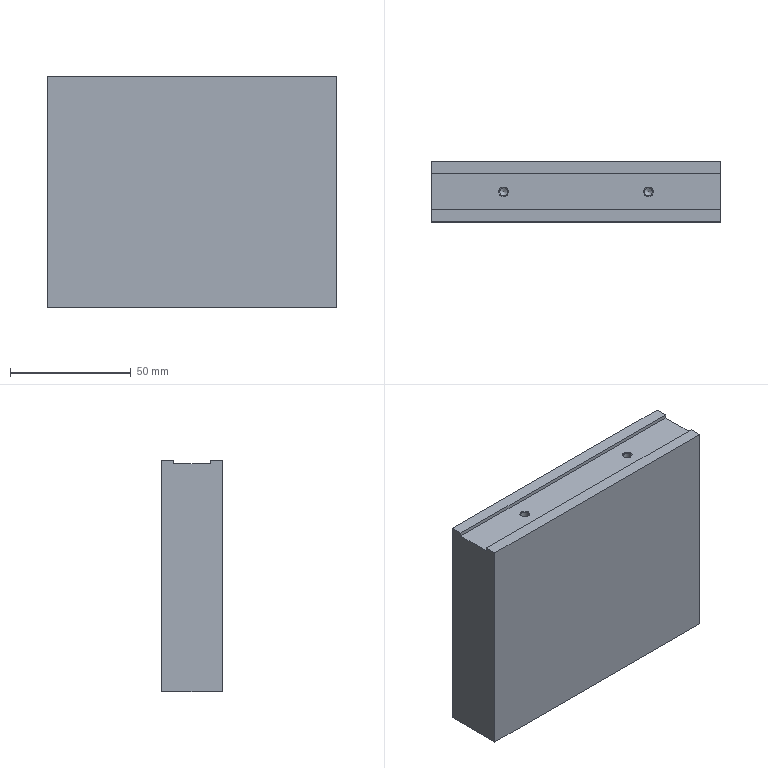Part | STEP file | Tube necking machine_id566_x_t | 1 solid | 16 faces | box 120 x 25 x 96 mm | volume 284951 mm3 | plane 10 | cone 4 | cylinder 2 | commonest cylinder face diameters 3.3 x2
STEP:
#1=CARTESIAN_POINT('',(0.,0.,0.));
#2=DIRECTION('',(0.,0.,1.));
#3=DIRECTION('',(1.,0.,0.));
#4=AXIS2_PLACEMENT_3D('',#1,#2,#3);
#5=CARTESIAN_POINT('',(210.,57.5,116.));
#6=VERTEX_POINT('',#5);
#7=CARTESIAN_POINT('',(210.,57.5,114.5));
#8=VERTEX_POINT('',#7);
#9=CARTESIAN_POINT('',(210.,57.5,115.681));
#10=DIRECTION('',(0.,0.,-1.));
#11=VECTOR('',#10,1.);
#12=LINE('',#9,#11);
#13=CARTESIAN_POINT('',(210.,62.5,136.));
#14=DIRECTION('',(1.,0.,0.));
#15=DIRECTION('',(0.,0.,-1.));
#16=AXIS2_PLACEMENT_3D('',#13,#14,#15);
#17=PLANE('',#16);
#18=CARTESIAN_POINT('',(20.319,-5.));
#19=DIRECTION('',(1.,0.));
#20=VECTOR('',#19,1.);
#21=LINE('',#18,#20);
#22=(GEOMETRIC_REPRESENTATION_CONTEXT(2)PARAMETRIC_REPRESENTATION_CONTEXT()REPRESENTATION_CONTEXT('',''));
#23=DEFINITIONAL_REPRESENTATION('',(#21),#22);
#24=PCURVE('',#17,#23);
#25=CARTESIAN_POINT('',(-741.73,57.5,115.681));
#26=DIRECTION('',(0.,1.,0.));
#27=DIRECTION('',(0.,0.,1.));
#28=AXIS2_PLACEMENT_3D('',#25,#26,#27);
#29=PLANE('',#28);
#30=CARTESIAN_POINT('',(0.,951.73));
#31=DIRECTION('',(-1.,0.));
#32=VECTOR('',#31,1.);
#33=LINE('',#30,#32);
#34=(GEOMETRIC_REPRESENTATION_CONTEXT(2)PARAMETRIC_REPRESENTATION_CONTEXT()REPRESENTATION_CONTEXT('',''));
#35=DEFINITIONAL_REPRESENTATION('',(#33),#34);
#36=PCURVE('',#29,#35);
#37=SURFACE_CURVE('',#12,(#24,#36),.PCURVE_S1.);
#38=EDGE_CURVE('',#6,#8,#37,.T.);
#39=ORIENTED_EDGE('',*,*,#38,.F.);
#40=CARTESIAN_POINT('',(210.,62.5,116.));
#41=VERTEX_POINT('',#40);
#42=CARTESIAN_POINT('',(210.,62.5,116.));
#43=DIRECTION('',(0.,-1.,0.));
#44=VECTOR('',#43,1.);
#45=LINE('',#42,#44);
#46=CARTESIAN_POINT('',(20.,0.));
#47=DIRECTION('',(0.,-1.));
#48=VECTOR('',#47,1.);
#49=LINE('',#46,#48);
#50=(GEOMETRIC_REPRESENTATION_CONTEXT(2)PARAMETRIC_REPRESENTATION_CONTEXT()REPRESENTATION_CONTEXT('',''));
#51=DEFINITIONAL_REPRESENTATION('',(#49),#50);
#52=PCURVE('',#17,#51);
#53=CARTESIAN_POINT('',(2.5,0.,116.));
#54=DIRECTION('',(0.,0.,1.));
#55=DIRECTION('',(1.,0.,0.));
#56=AXIS2_PLACEMENT_3D('',#53,#54,#55);
#57=PLANE('',#56);
#58=CARTESIAN_POINT('',(207.5,62.5));
#59=DIRECTION('',(0.,-1.));
#60=VECTOR('',#59,1.);
#61=LINE('',#58,#60);
#62=(GEOMETRIC_REPRESENTATION_CONTEXT(2)PARAMETRIC_REPRESENTATION_CONTEXT()REPRESENTATION_CONTEXT('',''));
#63=DEFINITIONAL_REPRESENTATION('',(#61),#62);
#64=PCURVE('',#57,#63);
#65=SURFACE_CURVE('',#45,(#52,#64),.PCURVE_S1.);
#66=EDGE_CURVE('',#41,#6,#65,.T.);
#67=ORIENTED_EDGE('',*,*,#66,.F.);
#68=CARTESIAN_POINT('',(210.,62.5,20.));
#69=VERTEX_POINT('',#68);
#70=CARTESIAN_POINT('',(210.,62.5,136.));
#71=DIRECTION('',(0.,0.,-1.));
#72=VECTOR('',#71,1.);
#73=LINE('',#70,#72);
#74=CARTESIAN_POINT('',(0.,0.));
#75=DIRECTION('',(1.,0.));
#76=VECTOR('',#75,1.);
#77=LINE('',#74,#76);
#78=(GEOMETRIC_REPRESENTATION_CONTEXT(2)PARAMETRIC_REPRESENTATION_CONTEXT()REPRESENTATION_CONTEXT('',''));
#79=DEFINITIONAL_REPRESENTATION('',(#77),#78);
#80=PCURVE('',#17,#79);
#81=CARTESIAN_POINT('',(330.,62.5,136.));
#82=DIRECTION('',(0.,-1.,0.));
#83=DIRECTION('',(0.,0.,-1.));
#84=AXIS2_PLACEMENT_3D('',#81,#82,#83);
#85=PLANE('',#84);
#86=CARTESIAN_POINT('',(0.,-120.));
#87=DIRECTION('',(1.,0.));
#88=VECTOR('',#87,1.);
#89=LINE('',#86,#88);
#90=(GEOMETRIC_REPRESENTATION_CONTEXT(2)PARAMETRIC_REPRESENTATION_CONTEXT()REPRESENTATION_CONTEXT('',''));
#91=DEFINITIONAL_REPRESENTATION('',(#89),#90);
#92=PCURVE('',#85,#91);
#93=SURFACE_CURVE('',#73,(#80,#92),.PCURVE_S1.);
#94=EDGE_CURVE('',#41,#69,#93,.T.);
#95=ORIENTED_EDGE('',*,*,#94,.T.);
#96=CARTESIAN_POINT('',(210.,37.5,20.));
#97=VERTEX_POINT('',#96);
#98=CARTESIAN_POINT('',(210.,62.5,20.));
#99=DIRECTION('',(0.,-1.,0.));
#100=VECTOR('',#99,1.);
#101=LINE('',#98,#100);
#102=CARTESIAN_POINT('',(116.,0.));
#103=DIRECTION('',(0.,-1.));
#104=VECTOR('',#103,1.);
#105=LINE('',#102,#104);
#106=(GEOMETRIC_REPRESENTATION_CONTEXT(2)PARAMETRIC_REPRESENTATION_CONTEXT()REPRESENTATION_CONTEXT('',''));
#107=DEFINITIONAL_REPRESENTATION('',(#105),#106);
#108=PCURVE('',#17,#107);
#109=CARTESIAN_POINT('',(2.5,0.,20.));
#110=DIRECTION('',(0.,0.,1.));
#111=DIRECTION('',(1.,0.,0.));
#112=AXIS2_PLACEMENT_3D('',#109,#110,#111);
#113=PLANE('',#112);
#114=CARTESIAN_POINT('',(207.5,62.5));
#115=DIRECTION('',(0.,-1.));
#116=VECTOR('',#115,1.);
#117=LINE('',#114,#116);
#118=(GEOMETRIC_REPRESENTATION_CONTEXT(2)PARAMETRIC_REPRESENTATION_CONTEXT()REPRESENTATION_CONTEXT('',''));
#119=DEFINITIONAL_REPRESENTATION('',(#117),#118);
#120=PCURVE('',#113,#119);
#121=SURFACE_CURVE('',#101,(#108,#120),.PCURVE_S1.);
#122=EDGE_CURVE('',#69,#97,#121,.T.);
#123=ORIENTED_EDGE('',*,*,#122,.T.);
#124=CARTESIAN_POINT('',(210.,37.5,116.));
#125=VERTEX_POINT('',#124);
#126=CARTESIAN_POINT('',(210.,37.5,136.));
#127=DIRECTION('',(0.,0.,-1.));
#128=VECTOR('',#127,1.);
#129=LINE('',#126,#128);
#130=CARTESIAN_POINT('',(0.,-25.));
#131=DIRECTION('',(1.,0.));
#132=VECTOR('',#131,1.);
#133=LINE('',#130,#132);
#134=(GEOMETRIC_REPRESENTATION_CONTEXT(2)PARAMETRIC_REPRESENTATION_CONTEXT()REPRESENTATION_CONTEXT('',''));
#135=DEFINITIONAL_REPRESENTATION('',(#133),#134);
#136=PCURVE('',#17,#135);
#137=CARTESIAN_POINT('',(210.,37.5,136.));
#138=DIRECTION('',(0.,1.,0.));
#139=DIRECTION('',(0.,0.,1.));
#140=AXIS2_PLACEMENT_3D('',#137,#138,#139);
#141=PLANE('',#140);
#142=CARTESIAN_POINT('',(0.,0.));
#143=DIRECTION('',(-1.,0.));
#144=VECTOR('',#143,1.);
#145=LINE('',#142,#144);
#146=(GEOMETRIC_REPRESENTATION_CONTEXT(2)PARAMETRIC_REPRESENTATION_CONTEXT()REPRESENTATION_CONTEXT('',''));
#147=DEFINITIONAL_REPRESENTATION('',(#145),#146);
#148=PCURVE('',#141,#147);
#149=SURFACE_CURVE('',#129,(#136,#148),.PCURVE_S1.);
#150=EDGE_CURVE('',#125,#97,#149,.T.);
#151=ORIENTED_EDGE('',*,*,#150,.F.);
#152=CARTESIAN_POINT('',(210.,42.5,116.));
#153=VERTEX_POINT('',#152);
#154=CARTESIAN_POINT('',(210.,62.5,116.));
#155=DIRECTION('',(0.,-1.,0.));
#156=VECTOR('',#155,1.);
#157=LINE('',#154,#156);
#158=CARTESIAN_POINT('',(20.,0.));
#159=DIRECTION('',(0.,-1.));
#160=VECTOR('',#159,1.);
#161=LINE('',#158,#160);
#162=(GEOMETRIC_REPRESENTATION_CONTEXT(2)PARAMETRIC_REPRESENTATION_CONTEXT()REPRESENTATION_CONTEXT('',''));
#163=DEFINITIONAL_REPRESENTATION('',(#161),#162);
#164=PCURVE('',#17,#163);
#165=CARTESIAN_POINT('',(2.5,0.,116.));
#166=DIRECTION('',(0.,0.,1.));
#167=DIRECTION('',(1.,0.,0.));
#168=AXIS2_PLACEMENT_3D('',#165,#166,#167);
#169=PLANE('',#168);
#170=CARTESIAN_POINT('',(207.5,62.5));
#171=DIRECTION('',(0.,-1.));
#172=VECTOR('',#171,1.);
#173=LINE('',#170,#172);
#174=(GEOMETRIC_REPRESENTATION_CONTEXT(2)PARAMETRIC_REPRESENTATION_CONTEXT()REPRESENTATION_CONTEXT('',''));
#175=DEFINITIONAL_REPRESENTATION('',(#173),#174);
#176=PCURVE('',#169,#175);
#177=SURFACE_CURVE('',#157,(#164,#176),.PCURVE_S1.);
#178=EDGE_CURVE('',#153,#125,#177,.T.);
#179=ORIENTED_EDGE('',*,*,#178,.F.);
#180=CARTESIAN_POINT('',(210.,42.5,114.5));
#181=VERTEX_POINT('',#180);
#182=CARTESIAN_POINT('',(210.,42.5,114.5));
#183=DIRECTION('',(0.,0.,1.));
#184=VECTOR('',#183,1.);
#185=LINE('',#182,#184);
#186=CARTESIAN_POINT('',(21.5,-20.));
#187=DIRECTION('',(-1.,0.));
#188=VECTOR('',#187,1.);
#189=LINE('',#186,#188);
#190=(GEOMETRIC_REPRESENTATION_CONTEXT(2)PARAMETRIC_REPRESENTATION_CONTEXT()REPRESENTATION_CONTEXT('',''));
#191=DEFINITIONAL_REPRESENTATION('',(#189),#190);
#192=PCURVE('',#17,#191);
#193=CARTESIAN_POINT('',(-741.73,42.5,114.5));
#194=DIRECTION('',(0.,-1.,0.));
#195=DIRECTION('',(0.,0.,-1.));
#196=AXIS2_PLACEMENT_3D('',#193,#194,#195);
#197=PLANE('',#196);
#198=CARTESIAN_POINT('',(0.,951.73));
#199=DIRECTION('',(-1.,0.));
#200=VECTOR('',#199,1.);
#201=LINE('',#198,#200);
#202=(GEOMETRIC_REPRESENTATION_CONTEXT(2)PARAMETRIC_REPRESENTATION_CONTEXT()REPRESENTATION_CONTEXT('',''));
#203=DEFINITIONAL_REPRESENTATION('',(#201),#202);
#204=PCURVE('',#197,#203);
#205=SURFACE_CURVE('',#185,(#192,#204),.PCURVE_S1.);
#206=EDGE_CURVE('',#181,#153,#205,.T.);
#207=ORIENTED_EDGE('',*,*,#206,.F.);
#208=CARTESIAN_POINT('',(210.,57.5,114.5));
#209=DIRECTION('',(0.,-1.,0.));
#210=VECTOR('',#209,1.);
#211=LINE('',#208,#210);
#212=CARTESIAN_POINT('',(21.5,-5.));
#213=DIRECTION('',(0.,-1.));
#214=VECTOR('',#213,1.);
#215=LINE('',#212,#214);
#216=(GEOMETRIC_REPRESENTATION_CONTEXT(2)PARAMETRIC_REPRESENTATION_CONTEXT()REPRESENTATION_CONTEXT('',''));
#217=DEFINITIONAL_REPRESENTATION('',(#215),#216);
#218=PCURVE('',#17,#217);
#219=CARTESIAN_POINT('',(-741.73,57.5,114.5));
#220=DIRECTION('',(0.,0.,-1.));
#221=DIRECTION('',(1.,0.,0.));
#222=AXIS2_PLACEMENT_3D('',#219,#220,#221);
#223=PLANE('',#222);
#224=CARTESIAN_POINT('',(951.73,0.));
#225=DIRECTION('',(0.,1.));
#226=VECTOR('',#225,1.);
#227=LINE('',#224,#226);
#228=(GEOMETRIC_REPRESENTATION_CONTEXT(2)PARAMETRIC_REPRESENTATION_CONTEXT()REPRESENTATION_CONTEXT('',''));
#229=DEFINITIONAL_REPRESENTATION('',(#227),#228);
#230=PCURVE('',#223,#229);
#231=SURFACE_CURVE('',#211,(#218,#230),.PCURVE_S1.);
#232=EDGE_CURVE('',#8,#181,#231,.T.);
#233=ORIENTED_EDGE('',*,*,#232,.F.);
#234=EDGE_LOOP('',(#39,#67,#95,#123,#151,#179,#207,#233));
#235=FACE_BOUND('',#234,.T.);
#236=ADVANCED_FACE('',(#235),#17,.F.);
#237=CARTESIAN_POINT('',(330.,42.5,116.));
#238=VERTEX_POINT('',#237);
#239=CARTESIAN_POINT('',(330.,42.5,114.5));
#240=VERTEX_POINT('',#239);
#241=CARTESIAN_POINT('',(330.,42.5,114.5));
#242=DIRECTION('',(0.,0.,-1.));
#243=VECTOR('',#242,1.);
#244=LINE('',#241,#243);
#245=CARTESIAN_POINT('',(330.,37.5,136.));
#246=DIRECTION('',(-1.,0.,0.));
#247=DIRECTION('',(0.,0.,1.));
#248=AXIS2_PLACEMENT_3D('',#245,#246,#247);
#249=PLANE('',#248);
#250=CARTESIAN_POINT('',(-21.5,5.));
#251=DIRECTION('',(-1.,0.));
#252=VECTOR('',#251,1.);
#253=LINE('',#250,#252);
#254=(GEOMETRIC_REPRESENTATION_CONTEXT(2)PARAMETRIC_REPRESENTATION_CONTEXT()REPRESENTATION_CONTEXT('',''));
#255=DEFINITIONAL_REPRESENTATION('',(#253),#254);
#256=PCURVE('',#249,#255);
#257=CARTESIAN_POINT('',(0.,1071.73));
#258=DIRECTION('',(1.,0.));
#259=VECTOR('',#258,1.);
#260=LINE('',#257,#259);
#261=(GEOMETRIC_REPRESENTATION_CONTEXT(2)PARAMETRIC_REPRESENTATION_CONTEXT()REPRESENTATION_CONTEXT('',''));
#262=DEFINITIONAL_REPRESENTATION('',(#260),#261);
#263=PCURVE('',#197,#262);
#264=SURFACE_CURVE('',#244,(#256,#263),.PCURVE_S1.);
#265=EDGE_CURVE('',#238,#240,#264,.T.);
#266=ORIENTED_EDGE('',*,*,#265,.F.);
#267=CARTESIAN_POINT('',(330.,37.5,116.));
#268=VERTEX_POINT('',#267);
#269=CARTESIAN_POINT('',(330.,37.5,116.));
#270=DIRECTION('',(0.,1.,0.));
#271=VECTOR('',#270,1.);
#272=LINE('',#269,#271);
#273=CARTESIAN_POINT('',(-20.,0.));
#274=DIRECTION('',(0.,1.));
#275=VECTOR('',#274,1.);
#276=LINE('',#273,#275);
#277=(GEOMETRIC_REPRESENTATION_CONTEXT(2)PARAMETRIC_REPRESENTATION_CONTEXT()REPRESENTATION_CONTEXT('',''));
#278=DEFINITIONAL_REPRESENTATION('',(#276),#277);
#279=PCURVE('',#249,#278);
#280=CARTESIAN_POINT('',(327.5,37.5));
#281=DIRECTION('',(0.,1.));
#282=VECTOR('',#281,1.);
#283=LINE('',#280,#282);
#284=(GEOMETRIC_REPRESENTATION_CONTEXT(2)PARAMETRIC_REPRESENTATION_CONTEXT()REPRESENTATION_CONTEXT('',''));
#285=DEFINITIONAL_REPRESENTATION('',(#283),#284);
#286=PCURVE('',#169,#285);
#287=SURFACE_CURVE('',#272,(#279,#286),.PCURVE_S1.);
#288=EDGE_CURVE('',#268,#238,#287,.T.);
#289=ORIENTED_EDGE('',*,*,#288,.F.);
#290=CARTESIAN_POINT('',(330.,37.5,20.));
#291=VERTEX_POINT('',#290);
#292=CARTESIAN_POINT('',(330.,37.5,136.));
#293=DIRECTION('',(0.,0.,-1.));
#294=VECTOR('',#293,1.);
#295=LINE('',#292,#294);
#296=CARTESIAN_POINT('',(0.,0.));
#297=DIRECTION('',(-1.,0.));
#298=VECTOR('',#297,1.);
#299=LINE('',#296,#298);
#300=(GEOMETRIC_REPRESENTATION_CONTEXT(2)PARAMETRIC_REPRESENTATION_CONTEXT()REPRESENTATION_CONTEXT('',''));
#301=DEFINITIONAL_REPRESENTATION('',(#299),#300);
#302=PCURVE('',#249,#301);
#303=CARTESIAN_POINT('',(0.,120.));
#304=DIRECTION('',(-1.,0.));
#305=VECTOR('',#304,1.);
#306=LINE('',#303,#305);
#307=(GEOMETRIC_REPRESENTATION_CONTEXT(2)PARAMETRIC_REPRESENTATION_CONTEXT()REPRESENTATION_CONTEXT('',''));
#308=DEFINITIONAL_REPRESENTATION('',(#306),#307);
#309=PCURVE('',#141,#308);
#310=SURFACE_CURVE('',#295,(#302,#309),.PCURVE_S1.);
#311=EDGE_CURVE('',#268,#291,#310,.T.);
#312=ORIENTED_EDGE('',*,*,#311,.T.);
#313=CARTESIAN_POINT('',(330.,62.5,20.));
#314=VERTEX_POINT('',#313);
#315=CARTESIAN_POINT('',(330.,37.5,20.));
#316=DIRECTION('',(0.,1.,0.));
#317=VECTOR('',#316,1.);
#318=LINE('',#315,#317);
#319=CARTESIAN_POINT('',(-116.,0.));
#320=DIRECTION('',(0.,1.));
#321=VECTOR('',#320,1.);
#322=LINE('',#319,#321);
#323=(GEOMETRIC_REPRESENTATION_CONTEXT(2)PARAMETRIC_REPRESENTATION_CONTEXT()REPRESENTATION_CONTEXT('',''));
#324=DEFINITIONAL_REPRESENTATION('',(#322),#323);
#325=PCURVE('',#249,#324);
#326=CARTESIAN_POINT('',(327.5,37.5));
#327=DIRECTION('',(0.,1.));
#328=VECTOR('',#327,1.);
#329=LINE('',#326,#328);
#330=(GEOMETRIC_REPRESENTATION_CONTEXT(2)PARAMETRIC_REPRESENTATION_CONTEXT()REPRESENTATION_CONTEXT('',''));
#331=DEFINITIONAL_REPRESENTATION('',(#329),#330);
#332=PCURVE('',#113,#331);
#333=SURFACE_CURVE('',#318,(#325,#332),.PCURVE_S1.);
#334=EDGE_CURVE('',#291,#314,#333,.T.);
#335=ORIENTED_EDGE('',*,*,#334,.T.);
#336=CARTESIAN_POINT('',(330.,62.5,116.));
#337=VERTEX_POINT('',#336);
#338=CARTESIAN_POINT('',(330.,62.5,136.));
#339=DIRECTION('',(0.,0.,-1.));
#340=VECTOR('',#339,1.);
#341=LINE('',#338,#340);
#342=CARTESIAN_POINT('',(0.,25.));
#343=DIRECTION('',(-1.,0.));
#344=VECTOR('',#343,1.);
#345=LINE('',#342,#344);
#346=(GEOMETRIC_REPRESENTATION_CONTEXT(2)PARAMETRIC_REPRESENTATION_CONTEXT()REPRESENTATION_CONTEXT('',''));
#347=DEFINITIONAL_REPRESENTATION('',(#345),#346);
#348=PCURVE('',#249,#347);
#349=CARTESIAN_POINT('',(0.,0.));
#350=DIRECTION('',(1.,0.));
#351=VECTOR('',#350,1.);
#352=LINE('',#349,#351);
#353=(GEOMETRIC_REPRESENTATION_CONTEXT(2)PARAMETRIC_REPRESENTATION_CONTEXT()REPRESENTATION_CONTEXT('',''));
#354=DEFINITIONAL_REPRESENTATION('',(#352),#353);
#355=PCURVE('',#85,#354);
#356=SURFACE_CURVE('',#341,(#348,#355),.PCURVE_S1.);
#357=EDGE_CURVE('',#337,#314,#356,.T.);
#358=ORIENTED_EDGE('',*,*,#357,.F.);
#359=CARTESIAN_POINT('',(330.,57.5,116.));
#360=VERTEX_POINT('',#359);
#361=CARTESIAN_POINT('',(330.,37.5,116.));
#362=DIRECTION('',(0.,1.,0.));
#363=VECTOR('',#362,1.);
#364=LINE('',#361,#363);
#365=CARTESIAN_POINT('',(-20.,0.));
#366=DIRECTION('',(0.,1.));
#367=VECTOR('',#366,1.);
#368=LINE('',#365,#367);
#369=(GEOMETRIC_REPRESENTATION_CONTEXT(2)PARAMETRIC_REPRESENTATION_CONTEXT()REPRESENTATION_CONTEXT('',''));
#370=DEFINITIONAL_REPRESENTATION('',(#368),#369);
#371=PCURVE('',#249,#370);
#372=CARTESIAN_POINT('',(327.5,37.5));
#373=DIRECTION('',(0.,1.));
#374=VECTOR('',#373,1.);
#375=LINE('',#372,#374);
#376=(GEOMETRIC_REPRESENTATION_CONTEXT(2)PARAMETRIC_REPRESENTATION_CONTEXT()REPRESENTATION_CONTEXT('',''));
#377=DEFINITIONAL_REPRESENTATION('',(#375),#376);
#378=PCURVE('',#57,#377);
#379=SURFACE_CURVE('',#364,(#371,#378),.PCURVE_S1.);
#380=EDGE_CURVE('',#360,#337,#379,.T.);
#381=ORIENTED_EDGE('',*,*,#380,.F.);
#382=CARTESIAN_POINT('',(330.,57.5,114.5));
#383=VERTEX_POINT('',#382);
#384=CARTESIAN_POINT('',(330.,57.5,115.681));
#385=DIRECTION('',(0.,0.,1.));
#386=VECTOR('',#385,1.);
#387=LINE('',#384,#386);
#388=CARTESIAN_POINT('',(-20.319,20.));
#389=DIRECTION('',(1.,0.));
#390=VECTOR('',#389,1.);
#391=LINE('',#388,#390);
#392=(GEOMETRIC_REPRESENTATION_CONTEXT(2)PARAMETRIC_REPRESENTATION_CONTEXT()REPRESENTATION_CONTEXT('',''));
#393=DEFINITIONAL_REPRESENTATION('',(#391),#392);
#394=PCURVE('',#249,#393);
#395=CARTESIAN_POINT('',(0.,1071.73));
#396=DIRECTION('',(1.,0.));
#397=VECTOR('',#396,1.);
#398=LINE('',#395,#397);
#399=(GEOMETRIC_REPRESENTATION_CONTEXT(2)PARAMETRIC_REPRESENTATION_CONTEXT()REPRESENTATION_CONTEXT('',''));
#400=DEFINITIONAL_REPRESENTATION('',(#398),#399);
#401=PCURVE('',#29,#400);
#402=SURFACE_CURVE('',#387,(#394,#401),.PCURVE_S1.);
#403=EDGE_CURVE('',#383,#360,#402,.T.);
#404=ORIENTED_EDGE('',*,*,#403,.F.);
#405=CARTESIAN_POINT('',(330.,57.5,114.5));
#406=DIRECTION('',(0.,1.,0.));
#407=VECTOR('',#406,1.);
#408=LINE('',#405,#407);
#409=CARTESIAN_POINT('',(-21.5,20.));
#410=DIRECTION('',(0.,1.));
#411=VECTOR('',#410,1.);
#412=LINE('',#409,#411);
#413=(GEOMETRIC_REPRESENTATION_CONTEXT(2)PARAMETRIC_REPRESENTATION_CONTEXT()REPRESENTATION_CONTEXT('',''));
#414=DEFINITIONAL_REPRESENTATION('',(#412),#413);
#415=PCURVE('',#249,#414);
#416=CARTESIAN_POINT('',(1071.73,0.));
#417=DIRECTION('',(0.,-1.));
#418=VECTOR('',#417,1.);
#419=LINE('',#416,#418);
#420=(GEOMETRIC_REPRESENTATION_CONTEXT(2)PARAMETRIC_REPRESENTATION_CONTEXT()REPRESENTATION_CONTEXT('',''));
#421=DEFINITIONAL_REPRESENTATION('',(#419),#420);
#422=PCURVE('',#223,#421);
#423=SURFACE_CURVE('',#408,(#415,#422),.PCURVE_S1.);
#424=EDGE_CURVE('',#240,#383,#423,.T.);
#425=ORIENTED_EDGE('',*,*,#424,.F.);
#426=EDGE_LOOP('',(#266,#289,#312,#335,#358,#381,#404,#425));
#427=FACE_BOUND('',#426,.T.);
#428=ADVANCED_FACE('',(#427),#249,.F.);
#429=CARTESIAN_POINT('',(2.5,42.5,116.));
#430=DIRECTION('',(1.,0.,0.));
#431=VECTOR('',#430,1.);
#432=LINE('',#429,#431);
#433=CARTESIAN_POINT('',(0.,42.5));
#434=DIRECTION('',(1.,0.));
#435=VECTOR('',#434,1.);
#436=LINE('',#433,#435);
#437=(GEOMETRIC_REPRESENTATION_CONTEXT(2)PARAMETRIC_REPRESENTATION_CONTEXT()REPRESENTATION_CONTEXT('',''));
#438=DEFINITIONAL_REPRESENTATION('',(#436),#437);
#439=PCURVE('',#169,#438);
#440=CARTESIAN_POINT('',(-1.5,744.23));
#441=DIRECTION('',(0.,1.));
#442=VECTOR('',#441,1.);
#443=LINE('',#440,#442);
#444=(GEOMETRIC_REPRESENTATION_CONTEXT(2)PARAMETRIC_REPRESENTATION_CONTEXT()REPRESENTATION_CONTEXT('',''));
#445=DEFINITIONAL_REPRESENTATION('',(#443),#444);
#446=PCURVE('',#197,#445);
#447=SURFACE_CURVE('',#432,(#439,#446),.PCURVE_S1.);
#448=EDGE_CURVE('',#153,#238,#447,.T.);
#449=ORIENTED_EDGE('',*,*,#448,.F.);
#450=ORIENTED_EDGE('',*,*,#178,.T.);
#451=CARTESIAN_POINT('',(210.,37.5,116.));
#452=DIRECTION('',(1.,0.,0.));
#453=VECTOR('',#452,1.);
#454=LINE('',#451,#453);
#455=CARTESIAN_POINT('',(207.5,37.5));
#456=DIRECTION('',(1.,0.));
#457=VECTOR('',#456,1.);
#458=LINE('',#455,#457);
#459=(GEOMETRIC_REPRESENTATION_CONTEXT(2)PARAMETRIC_REPRESENTATION_CONTEXT()REPRESENTATION_CONTEXT('',''));
#460=DEFINITIONAL_REPRESENTATION('',(#458),#459);
#461=PCURVE('',#169,#460);
#462=CARTESIAN_POINT('',(-20.,0.));
#463=DIRECTION('',(0.,1.));
#464=VECTOR('',#463,1.);
#465=LINE('',#462,#464);
#466=(GEOMETRIC_REPRESENTATION_CONTEXT(2)PARAMETRIC_REPRESENTATION_CONTEXT()REPRESENTATION_CONTEXT('',''));
#467=DEFINITIONAL_REPRESENTATION('',(#465),#466);
#468=PCURVE('',#141,#467);
#469=SURFACE_CURVE('',#454,(#461,#468),.PCURVE_S1.);
#470=EDGE_CURVE('',#125,#268,#469,.T.);
#471=ORIENTED_EDGE('',*,*,#470,.T.);
#472=ORIENTED_EDGE('',*,*,#288,.T.);
#473=EDGE_LOOP('',(#449,#450,#471,#472));
#474=FACE_BOUND('',#473,.T.);
#475=ADVANCED_FACE('',(#474),#169,.T.);
#476=ORIENTED_EDGE('',*,*,#470,.F.);
#477=ORIENTED_EDGE('',*,*,#150,.T.);
#478=CARTESIAN_POINT('',(210.,37.5,20.));
#479=DIRECTION('',(1.,0.,0.));
#480=VECTOR('',#479,1.);
#481=LINE('',#478,#480);
#482=CARTESIAN_POINT('',(-116.,0.));
#483=DIRECTION('',(0.,1.));
#484=VECTOR('',#483,1.);
#485=LINE('',#482,#484);
#486=(GEOMETRIC_REPRESENTATION_CONTEXT(2)PARAMETRIC_REPRESENTATION_CONTEXT()REPRESENTATION_CONTEXT('',''));
#487=DEFINITIONAL_REPRESENTATION('',(#485),#486);
#488=PCURVE('',#141,#487);
#489=CARTESIAN_POINT('',(207.5,37.5));
#490=DIRECTION('',(1.,0.));
#491=VECTOR('',#490,1.);
#492=LINE('',#489,#491);
#493=(GEOMETRIC_REPRESENTATION_CONTEXT(2)PARAMETRIC_REPRESENTATION_CONTEXT()REPRESENTATION_CONTEXT('',''));
#494=DEFINITIONAL_REPRESENTATION('',(#492),#493);
#495=PCURVE('',#113,#494);
#496=SURFACE_CURVE('',#481,(#488,#495),.PCURVE_S1.);
#497=EDGE_CURVE('',#97,#291,#496,.T.);
#498=ORIENTED_EDGE('',*,*,#497,.T.);
#499=ORIENTED_EDGE('',*,*,#311,.F.);
#500=EDGE_LOOP('',(#476,#477,#498,#499));
#501=FACE_BOUND('',#500,.T.);
#502=ADVANCED_FACE('',(#501),#141,.F.);
#503=CARTESIAN_POINT('',(330.,62.5,116.));
#504=DIRECTION('',(-1.,0.,0.));
#505=VECTOR('',#504,1.);
#506=LINE('',#503,#505);
#507=CARTESIAN_POINT('',(20.,0.));
#508=DIRECTION('',(0.,-1.));
#509=VECTOR('',#508,1.);
#510=LINE('',#507,#509);
#511=(GEOMETRIC_REPRESENTATION_CONTEXT(2)PARAMETRIC_REPRESENTATION_CONTEXT()REPRESENTATION_CONTEXT('',''));
#512=DEFINITIONAL_REPRESENTATION('',(#510),#511);
#513=PCURVE('',#85,#512);
#514=CARTESIAN_POINT('',(327.5,62.5));
#515=DIRECTION('',(-1.,0.));
#516=VECTOR('',#515,1.);
#517=LINE('',#514,#516);
#518=(GEOMETRIC_REPRESENTATION_CONTEXT(2)PARAMETRIC_REPRESENTATION_CONTEXT()REPRESENTATION_CONTEXT('',''));
#519=DEFINITIONAL_REPRESENTATION('',(#517),#518);
#520=PCURVE('',#57,#519);
#521=SURFACE_CURVE('',#506,(#513,#520),.PCURVE_S1.);
#522=EDGE_CURVE('',#337,#41,#521,.T.);
#523=ORIENTED_EDGE('',*,*,#522,.F.);
#524=ORIENTED_EDGE('',*,*,#357,.T.);
#525=CARTESIAN_POINT('',(330.,62.5,20.));
#526=DIRECTION('',(-1.,0.,0.));
#527=VECTOR('',#526,1.);
#528=LINE('',#525,#527);
#529=CARTESIAN_POINT('',(116.,0.));
#530=DIRECTION('',(0.,-1.));
#531=VECTOR('',#530,1.);
#532=LINE('',#529,#531);
#533=(GEOMETRIC_REPRESENTATION_CONTEXT(2)PARAMETRIC_REPRESENTATION_CONTEXT()REPRESENTATION_CONTEXT('',''));
#534=DEFINITIONAL_REPRESENTATION('',(#532),#533);
#535=PCURVE('',#85,#534);
#536=CARTESIAN_POINT('',(327.5,62.5));
#537=DIRECTION('',(-1.,0.));
#538=VECTOR('',#537,1.);
#539=LINE('',#536,#538);
#540=(GEOMETRIC_REPRESENTATION_CONTEXT(2)PARAMETRIC_REPRESENTATION_CONTEXT()REPRESENTATION_CONTEXT('',''));
#541=DEFINITIONAL_REPRESENTATION('',(#539),#540);
#542=PCURVE('',#113,#541);
#543=SURFACE_CURVE('',#528,(#535,#542),.PCURVE_S1.);
#544=EDGE_CURVE('',#314,#69,#543,.T.);
#545=ORIENTED_EDGE('',*,*,#544,.T.);
#546=ORIENTED_EDGE('',*,*,#94,.F.);
#547=EDGE_LOOP('',(#523,#524,#545,#546));
#548=FACE_BOUND('',#547,.T.);
#549=ADVANCED_FACE('',(#548),#85,.F.);
#550=ORIENTED_EDGE('',*,*,#122,.F.);
#551=ORIENTED_EDGE('',*,*,#544,.F.);
#552=ORIENTED_EDGE('',*,*,#334,.F.);
#553=ORIENTED_EDGE('',*,*,#497,.F.);
#554=EDGE_LOOP('',(#550,#551,#552,#553));
#555=FACE_BOUND('',#554,.T.);
#556=ADVANCED_FACE('',(#555),#113,.F.);
#557=CARTESIAN_POINT('',(2.5,57.5,116.));
#558=DIRECTION('',(-1.,0.,0.));
#559=VECTOR('',#558,1.);
#560=LINE('',#557,#559);
#561=CARTESIAN_POINT('',(0.,57.5));
#562=DIRECTION('',(-1.,0.));
#563=VECTOR('',#562,1.);
#564=LINE('',#561,#563);
#565=(GEOMETRIC_REPRESENTATION_CONTEXT(2)PARAMETRIC_REPRESENTATION_CONTEXT()REPRESENTATION_CONTEXT('',''));
#566=DEFINITIONAL_REPRESENTATION('',(#564),#565);
#567=PCURVE('',#57,#566);
#568=CARTESIAN_POINT('',(0.3185,744.23));
#569=DIRECTION('',(0.,-1.));
#570=VECTOR('',#569,1.);
#571=LINE('',#568,#570);
#572=(GEOMETRIC_REPRESENTATION_CONTEXT(2)PARAMETRIC_REPRESENTATION_CONTEXT()REPRESENTATION_CONTEXT('',''));
#573=DEFINITIONAL_REPRESENTATION('',(#571),#572);
#574=PCURVE('',#29,#573);
#575=SURFACE_CURVE('',#560,(#567,#574),.PCURVE_S1.);
#576=EDGE_CURVE('',#360,#6,#575,.T.);
#577=ORIENTED_EDGE('',*,*,#576,.F.);
#578=ORIENTED_EDGE('',*,*,#380,.T.);
#579=ORIENTED_EDGE('',*,*,#522,.T.);
#580=ORIENTED_EDGE('',*,*,#66,.T.);
#581=EDGE_LOOP('',(#577,#578,#579,#580));
#582=FACE_BOUND('',#581,.T.);
#583=ADVANCED_FACE('',(#582),#57,.T.);
#584=ORIENTED_EDGE('',*,*,#448,.T.);
#585=ORIENTED_EDGE('',*,*,#265,.T.);
#586=CARTESIAN_POINT('',(-741.73,42.5,114.5));
#587=DIRECTION('',(1.,0.,0.));
#588=VECTOR('',#587,1.);
#589=LINE('',#586,#588);
#590=CARTESIAN_POINT('',(0.,0.));
#591=DIRECTION('',(0.,1.));
#592=VECTOR('',#591,1.);
#593=LINE('',#590,#592);
#594=(GEOMETRIC_REPRESENTATION_CONTEXT(2)PARAMETRIC_REPRESENTATION_CONTEXT()REPRESENTATION_CONTEXT('',''));
#595=DEFINITIONAL_REPRESENTATION('',(#593),#594);
#596=PCURVE('',#197,#595);
#597=CARTESIAN_POINT('',(0.,15.));
#598=DIRECTION('',(1.,0.));
#599=VECTOR('',#598,1.);
#600=LINE('',#597,#599);
#601=(GEOMETRIC_REPRESENTATION_CONTEXT(2)PARAMETRIC_REPRESENTATION_CONTEXT()REPRESENTATION_CONTEXT('',''));
#602=DEFINITIONAL_REPRESENTATION('',(#600),#601);
#603=PCURVE('',#223,#602);
#604=SURFACE_CURVE('',#589,(#596,#603),.PCURVE_S1.);
#605=EDGE_CURVE('',#181,#240,#604,.T.);
#606=ORIENTED_EDGE('',*,*,#605,.F.);
#607=ORIENTED_EDGE('',*,*,#206,.T.);
#608=EDGE_LOOP('',(#584,#585,#606,#607));
#609=FACE_BOUND('',#608,.T.);
#610=ADVANCED_FACE('',(#609),#197,.F.);
#611=ORIENTED_EDGE('',*,*,#576,.T.);
#612=ORIENTED_EDGE('',*,*,#38,.T.);
#613=CARTESIAN_POINT('',(-741.73,57.5,114.5));
#614=DIRECTION('',(1.,0.,0.));
#615=VECTOR('',#614,1.);
#616=LINE('',#613,#615);
#617=CARTESIAN_POINT('',(-1.181,0.));
#618=DIRECTION('',(0.,1.));
#619=VECTOR('',#618,1.);
#620=LINE('',#617,#619);
#621=(GEOMETRIC_REPRESENTATION_CONTEXT(2)PARAMETRIC_REPRESENTATION_CONTEXT()REPRESENTATION_CONTEXT('',''));
#622=DEFINITIONAL_REPRESENTATION('',(#620),#621);
#623=PCURVE('',#29,#622);
#624=CARTESIAN_POINT('',(0.,0.));
#625=DIRECTION('',(1.,0.));
#626=VECTOR('',#625,1.);
#627=LINE('',#624,#626);
#628=(GEOMETRIC_REPRESENTATION_CONTEXT(2)PARAMETRIC_REPRESENTATION_CONTEXT()REPRESENTATION_CONTEXT('',''));
#629=DEFINITIONAL_REPRESENTATION('',(#627),#628);
#630=PCURVE('',#223,#629);
#631=SURFACE_CURVE('',#616,(#623,#630),.PCURVE_S1.);
#632=EDGE_CURVE('',#8,#383,#631,.T.);
#633=ORIENTED_EDGE('',*,*,#632,.T.);
#634=ORIENTED_EDGE('',*,*,#403,.T.);
#635=EDGE_LOOP('',(#611,#612,#633,#634));
#636=FACE_BOUND('',#635,.T.);
#637=ADVANCED_FACE('',(#636),#29,.F.);
#638=CARTESIAN_POINT('',(298.,50.,114.5));
#639=VERTEX_POINT('',#638);
#640=CARTESIAN_POINT('',(300.,50.,114.5));
#641=DIRECTION('',(0.,0.,-1.));
#642=DIRECTION('',(-1.,0.,0.));
#643=AXIS2_PLACEMENT_3D('',#640,#641,#642);
#644=CIRCLE('',#643,2.);
#645=CARTESIAN_POINT('',(1041.73,7.5));
#646=DIRECTION('',(-1.,0.));
#647=AXIS2_PLACEMENT_2D('',#645,#646);
#648=CIRCLE('',#647,2.);
#649=(GEOMETRIC_REPRESENTATION_CONTEXT(2)PARAMETRIC_REPRESENTATION_CONTEXT()REPRESENTATION_CONTEXT('',''));
#650=DEFINITIONAL_REPRESENTATION('',(#648),#649);
#651=PCURVE('',#223,#650);
#652=CARTESIAN_POINT('',(300.,50.,114.5));
#653=DIRECTION('',(0.,0.,1.));
#654=DIRECTION('',(1.,0.,0.));
#655=AXIS2_PLACEMENT_3D('',#652,#653,#654);
#656=CONICAL_SURFACE('',#655,2.,0.7854);
#657=CARTESIAN_POINT('',(9.425,0.));
#658=DIRECTION('',(-1.,0.));
#659=VECTOR('',#658,1.);
#660=LINE('',#657,#659);
#661=(GEOMETRIC_REPRESENTATION_CONTEXT(2)PARAMETRIC_REPRESENTATION_CONTEXT()REPRESENTATION_CONTEXT('',''));
#662=DEFINITIONAL_REPRESENTATION('',(#660),#661);
#663=PCURVE('',#656,#662);
#664=SURFACE_CURVE('',#644,(#651,#663),.PCURVE_S1.);
#665=EDGE_CURVE('',#639,#639,#664,.T.);
#666=ORIENTED_EDGE('',*,*,#665,.T.);
#667=EDGE_LOOP('',(#666));
#668=FACE_BOUND('',#667,.T.);
#669=CARTESIAN_POINT('',(238.,50.,114.5));
#670=VERTEX_POINT('',#669);
#671=CARTESIAN_POINT('',(240.,50.,114.5));
#672=DIRECTION('',(0.,0.,-1.));
#673=DIRECTION('',(-1.,0.,0.));
#674=AXIS2_PLACEMENT_3D('',#671,#672,#673);
#675=CIRCLE('',#674,2.);
#676=CARTESIAN_POINT('',(981.73,7.5));
#677=DIRECTION('',(-1.,0.));
#678=AXIS2_PLACEMENT_2D('',#676,#677);
#679=CIRCLE('',#678,2.);
#680=(GEOMETRIC_REPRESENTATION_CONTEXT(2)PARAMETRIC_REPRESENTATION_CONTEXT()REPRESENTATION_CONTEXT('',''));
#681=DEFINITIONAL_REPRESENTATION('',(#679),#680);
#682=PCURVE('',#223,#681);
#683=CARTESIAN_POINT('',(240.,50.,114.5));
#684=DIRECTION('',(0.,0.,1.));
#685=DIRECTION('',(1.,0.,0.));
#686=AXIS2_PLACEMENT_3D('',#683,#684,#685);
#687=CONICAL_SURFACE('',#686,2.,0.7854);
#688=CARTESIAN_POINT('',(9.425,0.));
#689=DIRECTION('',(-1.,0.));
#690=VECTOR('',#689,1.);
#691=LINE('',#688,#690);
#692=(GEOMETRIC_REPRESENTATION_CONTEXT(2)PARAMETRIC_REPRESENTATION_CONTEXT()REPRESENTATION_CONTEXT('',''));
#693=DEFINITIONAL_REPRESENTATION('',(#691),#692);
#694=PCURVE('',#687,#693);
#695=SURFACE_CURVE('',#675,(#682,#694),.PCURVE_S1.);
#696=EDGE_CURVE('',#670,#670,#695,.T.);
#697=ORIENTED_EDGE('',*,*,#696,.T.);
#698=EDGE_LOOP('',(#697));
#699=FACE_BOUND('',#698,.T.);
#700=ORIENTED_EDGE('',*,*,#232,.T.);
#701=ORIENTED_EDGE('',*,*,#605,.T.);
#702=ORIENTED_EDGE('',*,*,#424,.T.);
#703=ORIENTED_EDGE('',*,*,#632,.F.);
#704=EDGE_LOOP('',(#700,#701,#702,#703));
#705=FACE_BOUND('',#704,.T.);
#706=ADVANCED_FACE('',(#668,#699,#705),#223,.F.);
#707=CARTESIAN_POINT('',(241.65,50.,94.5));
#708=VERTEX_POINT('',#707);
#709=CARTESIAN_POINT('',(238.35,50.,94.5));
#710=VERTEX_POINT('',#709);
#711=CARTESIAN_POINT('',(240.,50.,94.5));
#712=DIRECTION('',(0.,0.,1.));
#713=DIRECTION('',(-1.,0.,0.));
#714=AXIS2_PLACEMENT_3D('',#711,#712,#713);
#715=CIRCLE('',#714,1.65);
#716=CARTESIAN_POINT('',(240.,50.,94.5));
#717=DIRECTION('',(0.,0.,1.));
#718=DIRECTION('',(1.,0.,0.));
#719=AXIS2_PLACEMENT_3D('',#716,#717,#718);
#720=CONICAL_SURFACE('',#719,1.65,1.03);
#721=CARTESIAN_POINT('',(-3.142,0.));
#722=DIRECTION('',(1.,0.));
#723=VECTOR('',#722,1.);
#724=LINE('',#721,#723);
#725=(GEOMETRIC_REPRESENTATION_CONTEXT(2)PARAMETRIC_REPRESENTATION_CONTEXT()REPRESENTATION_CONTEXT('',''));
#726=DEFINITIONAL_REPRESENTATION('',(#724),#725);
#727=PCURVE('',#720,#726);
#728=CARTESIAN_POINT('',(240.,50.,114.5));
#729=DIRECTION('',(0.,0.,-1.));
#730=DIRECTION('',(-1.,0.,0.));
#731=AXIS2_PLACEMENT_3D('',#728,#729,#730);
#732=CYLINDRICAL_SURFACE('',#731,1.65);
#733=CARTESIAN_POINT('',(6.283,20.));
#734=DIRECTION('',(-1.,0.));
#735=VECTOR('',#734,1.);
#736=LINE('',#733,#735);
#737=(GEOMETRIC_REPRESENTATION_CONTEXT(2)PARAMETRIC_REPRESENTATION_CONTEXT()REPRESENTATION_CONTEXT('',''));
#738=DEFINITIONAL_REPRESENTATION('',(#736),#737);
#739=PCURVE('',#732,#738);
#740=SURFACE_CURVE('',#715,(#727,#739),.PCURVE_S1.);
#741=EDGE_CURVE('',#708,#710,#740,.T.);
#742=ORIENTED_EDGE('',*,*,#741,.F.);
#743=CARTESIAN_POINT('',(240.,50.,93.509));
#744=VERTEX_POINT('',#743);
#745=CARTESIAN_POINT('',(240.,50.,93.509));
#746=CARTESIAN_POINT('',(241.65,50.,94.5));
#747=B_SPLINE_CURVE_WITH_KNOTS('',1,(#745,#746),.UNSPECIFIED.,.F.,.F.,(2,2),(-1.925,0.),.PIECEWISE_BEZIER_KNOTS.);
#748=CARTESIAN_POINT('',(0.,0.));
#749=DIRECTION('',(0.,1.));
#750=VECTOR('',#749,1.);
#751=LINE('',#748,#750);
#752=(GEOMETRIC_REPRESENTATION_CONTEXT(2)PARAMETRIC_REPRESENTATION_CONTEXT()REPRESENTATION_CONTEXT('',''));
#753=DEFINITIONAL_REPRESENTATION('',(#751),#752);
#754=PCURVE('',#720,#753);
#755=CARTESIAN_POINT('',(6.283,0.));
#756=DIRECTION('',(0.,1.));
#757=VECTOR('',#756,1.);
#758=LINE('',#755,#757);
#759=(GEOMETRIC_REPRESENTATION_CONTEXT(2)PARAMETRIC_REPRESENTATION_CONTEXT()REPRESENTATION_CONTEXT('',''));
#760=DEFINITIONAL_REPRESENTATION('',(#758),#759);
#761=PCURVE('',#720,#760);
#762=SEAM_CURVE('',#747,(#754,#761),.PCURVE_S1.);
#763=EDGE_CURVE('',#744,#708,#762,.T.);
#764=ORIENTED_EDGE('',*,*,#763,.F.);
#765=ORIENTED_EDGE('',*,*,#763,.T.);
#766=CARTESIAN_POINT('',(240.,50.,94.5));
#767=DIRECTION('',(0.,0.,1.));
#768=DIRECTION('',(-1.,0.,0.));
#769=AXIS2_PLACEMENT_3D('',#766,#767,#768);
#770=CIRCLE('',#769,1.65);
#771=CARTESIAN_POINT('',(3.142,0.));
#772=DIRECTION('',(1.,0.));
#773=VECTOR('',#772,1.);
#774=LINE('',#771,#773);
#775=(GEOMETRIC_REPRESENTATION_CONTEXT(2)PARAMETRIC_REPRESENTATION_CONTEXT()REPRESENTATION_CONTEXT('',''));
#776=DEFINITIONAL_REPRESENTATION('',(#774),#775);
#777=PCURVE('',#720,#776);
#778=CARTESIAN_POINT('',(6.283,20.));
#779=DIRECTION('',(-1.,0.));
#780=VECTOR('',#779,1.);
#781=LINE('',#778,#780);
#782=(GEOMETRIC_REPRESENTATION_CONTEXT(2)PARAMETRIC_REPRESENTATION_CONTEXT()REPRESENTATION_CONTEXT('',''));
#783=DEFINITIONAL_REPRESENTATION('',(#781),#782);
#784=PCURVE('',#732,#783);
#785=SURFACE_CURVE('',#770,(#777,#784),.PCURVE_S1.);
#786=EDGE_CURVE('',#710,#708,#785,.T.);
#787=ORIENTED_EDGE('',*,*,#786,.F.);
#788=EDGE_LOOP('',(#742,#764,#765,#787));
#789=FACE_BOUND('',#788,.F.);
#790=ADVANCED_FACE('',(#789),#720,.F.);
#791=CARTESIAN_POINT('',(238.35,50.,114.15));
#792=VERTEX_POINT('',#791);
#793=CARTESIAN_POINT('',(240.,50.,114.15));
#794=DIRECTION('',(0.,0.,1.));
#795=DIRECTION('',(-1.,0.,0.));
#796=AXIS2_PLACEMENT_3D('',#793,#794,#795);
#797=CIRCLE('',#796,1.65);
#798=CARTESIAN_POINT('',(6.283,0.35));
#799=DIRECTION('',(-1.,0.));
#800=VECTOR('',#799,1.);
#801=LINE('',#798,#800);
#802=(GEOMETRIC_REPRESENTATION_CONTEXT(2)PARAMETRIC_REPRESENTATION_CONTEXT()REPRESENTATION_CONTEXT('',''));
#803=DEFINITIONAL_REPRESENTATION('',(#801),#802);
#804=PCURVE('',#732,#803);
#805=CARTESIAN_POINT('',(3.142,-0.35));
#806=DIRECTION('',(1.,0.));
#807=VECTOR('',#806,1.);
#808=LINE('',#805,#807);
#809=(GEOMETRIC_REPRESENTATION_CONTEXT(2)PARAMETRIC_REPRESENTATION_CONTEXT()REPRESENTATION_CONTEXT('',''));
#810=DEFINITIONAL_REPRESENTATION('',(#808),#809);
#811=PCURVE('',#687,#810);
#812=SURFACE_CURVE('',#797,(#804,#811),.PCURVE_S1.);
#813=EDGE_CURVE('',#792,#792,#812,.T.);
#814=ORIENTED_EDGE('',*,*,#813,.F.);
#815=CARTESIAN_POINT('',(238.35,50.,114.15));
#816=CARTESIAN_POINT('',(238.35,50.,94.5));
#817=B_SPLINE_CURVE_WITH_KNOTS('',1,(#815,#816),.UNSPECIFIED.,.F.,.F.,(2,2),(0.35,20.),.PIECEWISE_BEZIER_KNOTS.);
#818=CARTESIAN_POINT('',(6.283,0.));
#819=DIRECTION('',(0.,1.));
#820=VECTOR('',#819,1.);
#821=LINE('',#818,#820);
#822=(GEOMETRIC_REPRESENTATION_CONTEXT(2)PARAMETRIC_REPRESENTATION_CONTEXT()REPRESENTATION_CONTEXT('',''));
#823=DEFINITIONAL_REPRESENTATION('',(#821),#822);
#824=PCURVE('',#732,#823);
#825=CARTESIAN_POINT('',(0.,0.));
#826=DIRECTION('',(0.,1.));
#827=VECTOR('',#826,1.);
#828=LINE('',#825,#827);
#829=(GEOMETRIC_REPRESENTATION_CONTEXT(2)PARAMETRIC_REPRESENTATION_CONTEXT()REPRESENTATION_CONTEXT('',''));
#830=DEFINITIONAL_REPRESENTATION('',(#828),#829);
#831=PCURVE('',#732,#830);
#832=SEAM_CURVE('',#817,(#824,#831),.PCURVE_S1.);
#833=EDGE_CURVE('',#792,#710,#832,.T.);
#834=ORIENTED_EDGE('',*,*,#833,.T.);
#835=ORIENTED_EDGE('',*,*,#786,.T.);
#836=ORIENTED_EDGE('',*,*,#741,.T.);
#837=ORIENTED_EDGE('',*,*,#833,.F.);
#838=EDGE_LOOP('',(#814,#834,#835,#836,#837));
#839=FACE_BOUND('',#838,.F.);
#840=ADVANCED_FACE('',(#839),#732,.F.);
#841=ORIENTED_EDGE('',*,*,#813,.T.);
#842=CARTESIAN_POINT('',(238.35,50.,114.15));
#843=CARTESIAN_POINT('',(238.,50.,114.5));
#844=B_SPLINE_CURVE_WITH_KNOTS('',1,(#842,#843),.UNSPECIFIED.,.F.,.F.,(2,2),(-0.495,0.),.PIECEWISE_BEZIER_KNOTS.);
#845=CARTESIAN_POINT('',(9.425,0.));
#846=DIRECTION('',(0.,1.));
#847=VECTOR('',#846,1.);
#848=LINE('',#845,#847);
#849=(GEOMETRIC_REPRESENTATION_CONTEXT(2)PARAMETRIC_REPRESENTATION_CONTEXT()REPRESENTATION_CONTEXT('',''));
#850=DEFINITIONAL_REPRESENTATION('',(#848),#849);
#851=PCURVE('',#687,#850);
#852=CARTESIAN_POINT('',(3.142,0.));
#853=DIRECTION('',(0.,1.));
#854=VECTOR('',#853,1.);
#855=LINE('',#852,#854);
#856=(GEOMETRIC_REPRESENTATION_CONTEXT(2)PARAMETRIC_REPRESENTATION_CONTEXT()REPRESENTATION_CONTEXT('',''));
#857=DEFINITIONAL_REPRESENTATION('',(#855),#856);
#858=PCURVE('',#687,#857);
#859=SEAM_CURVE('',#844,(#851,#858),.PCURVE_S1.);
#860=EDGE_CURVE('',#792,#670,#859,.T.);
#861=ORIENTED_EDGE('',*,*,#860,.T.);
#862=ORIENTED_EDGE('',*,*,#696,.T.);
#863=ORIENTED_EDGE('',*,*,#860,.F.);
#864=EDGE_LOOP('',(#841,#861,#862,#863));
#865=FACE_BOUND('',#864,.F.);
#866=ADVANCED_FACE('',(#865),#687,.F.);
#867=CARTESIAN_POINT('',(301.65,50.,94.5));
#868=VERTEX_POINT('',#867);
#869=CARTESIAN_POINT('',(298.35,50.,94.5));
#870=VERTEX_POINT('',#869);
#871=CARTESIAN_POINT('',(300.,50.,94.5));
#872=DIRECTION('',(0.,0.,1.));
#873=DIRECTION('',(-1.,0.,0.));
#874=AXIS2_PLACEMENT_3D('',#871,#872,#873);
#875=CIRCLE('',#874,1.65);
#876=CARTESIAN_POINT('',(300.,50.,94.5));
#877=DIRECTION('',(0.,0.,1.));
#878=DIRECTION('',(1.,0.,0.));
#879=AXIS2_PLACEMENT_3D('',#876,#877,#878);
#880=CONICAL_SURFACE('',#879,1.65,1.03);
#881=CARTESIAN_POINT('',(-3.142,0.));
#882=DIRECTION('',(1.,0.));
#883=VECTOR('',#882,1.);
#884=LINE('',#881,#883);
#885=(GEOMETRIC_REPRESENTATION_CONTEXT(2)PARAMETRIC_REPRESENTATION_CONTEXT()REPRESENTATION_CONTEXT('',''));
#886=DEFINITIONAL_REPRESENTATION('',(#884),#885);
#887=PCURVE('',#880,#886);
#888=CARTESIAN_POINT('',(300.,50.,114.5));
#889=DIRECTION('',(0.,0.,-1.));
#890=DIRECTION('',(-1.,0.,0.));
#891=AXIS2_PLACEMENT_3D('',#888,#889,#890);
#892=CYLINDRICAL_SURFACE('',#891,1.65);
#893=CARTESIAN_POINT('',(6.283,20.));
#894=DIRECTION('',(-1.,0.));
#895=VECTOR('',#894,1.);
#896=LINE('',#893,#895);
#897=(GEOMETRIC_REPRESENTATION_CONTEXT(2)PARAMETRIC_REPRESENTATION_CONTEXT()REPRESENTATION_CONTEXT('',''));
#898=DEFINITIONAL_REPRESENTATION('',(#896),#897);
#899=PCURVE('',#892,#898);
#900=SURFACE_CURVE('',#875,(#887,#899),.PCURVE_S1.);
#901=EDGE_CURVE('',#868,#870,#900,.T.);
#902=ORIENTED_EDGE('',*,*,#901,.F.);
#903=CARTESIAN_POINT('',(300.,50.,93.509));
#904=VERTEX_POINT('',#903);
#905=CARTESIAN_POINT('',(300.,50.,93.509));
#906=CARTESIAN_POINT('',(301.65,50.,94.5));
#907=B_SPLINE_CURVE_WITH_KNOTS('',1,(#905,#906),.UNSPECIFIED.,.F.,.F.,(2,2),(-1.925,0.),.PIECEWISE_BEZIER_KNOTS.);
#908=CARTESIAN_POINT('',(0.,0.));
#909=DIRECTION('',(0.,1.));
#910=VECTOR('',#909,1.);
#911=LINE('',#908,#910);
#912=(GEOMETRIC_REPRESENTATION_CONTEXT(2)PARAMETRIC_REPRESENTATION_CONTEXT()REPRESENTATION_CONTEXT('',''));
#913=DEFINITIONAL_REPRESENTATION('',(#911),#912);
#914=PCURVE('',#880,#913);
#915=CARTESIAN_POINT('',(6.283,0.));
#916=DIRECTION('',(0.,1.));
#917=VECTOR('',#916,1.);
#918=LINE('',#915,#917);
#919=(GEOMETRIC_REPRESENTATION_CONTEXT(2)PARAMETRIC_REPRESENTATION_CONTEXT()REPRESENTATION_CONTEXT('',''));
#920=DEFINITIONAL_REPRESENTATION('',(#918),#919);
#921=PCURVE('',#880,#920);
#922=SEAM_CURVE('',#907,(#914,#921),.PCURVE_S1.);
#923=EDGE_CURVE('',#904,#868,#922,.T.);
#924=ORIENTED_EDGE('',*,*,#923,.F.);
#925=ORIENTED_EDGE('',*,*,#923,.T.);
#926=CARTESIAN_POINT('',(300.,50.,94.5));
#927=DIRECTION('',(0.,0.,1.));
#928=DIRECTION('',(-1.,0.,0.));
#929=AXIS2_PLACEMENT_3D('',#926,#927,#928);
#930=CIRCLE('',#929,1.65);
#931=CARTESIAN_POINT('',(3.142,0.));
#932=DIRECTION('',(1.,0.));
#933=VECTOR('',#932,1.);
#934=LINE('',#931,#933);
#935=(GEOMETRIC_REPRESENTATION_CONTEXT(2)PARAMETRIC_REPRESENTATION_CONTEXT()REPRESENTATION_CONTEXT('',''));
#936=DEFINITIONAL_REPRESENTATION('',(#934),#935);
#937=PCURVE('',#880,#936);
#938=CARTESIAN_POINT('',(6.283,20.));
#939=DIRECTION('',(-1.,0.));
#940=VECTOR('',#939,1.);
#941=LINE('',#938,#940);
#942=(GEOMETRIC_REPRESENTATION_CONTEXT(2)PARAMETRIC_REPRESENTATION_CONTEXT()REPRESENTATION_CONTEXT('',''));
#943=DEFINITIONAL_REPRESENTATION('',(#941),#942);
#944=PCURVE('',#892,#943);
#945=SURFACE_CURVE('',#930,(#937,#944),.PCURVE_S1.);
#946=EDGE_CURVE('',#870,#868,#945,.T.);
#947=ORIENTED_EDGE('',*,*,#946,.F.);
#948=EDGE_LOOP('',(#902,#924,#925,#947));
#949=FACE_BOUND('',#948,.F.);
#950=ADVANCED_FACE('',(#949),#880,.F.);
#951=CARTESIAN_POINT('',(298.35,50.,114.15));
#952=VERTEX_POINT('',#951);
#953=CARTESIAN_POINT('',(300.,50.,114.15));
#954=DIRECTION('',(0.,0.,1.));
#955=DIRECTION('',(-1.,0.,0.));
#956=AXIS2_PLACEMENT_3D('',#953,#954,#955);
#957=CIRCLE('',#956,1.65);
#958=CARTESIAN_POINT('',(6.283,0.35));
#959=DIRECTION('',(-1.,0.));
#960=VECTOR('',#959,1.);
#961=LINE('',#958,#960);
#962=(GEOMETRIC_REPRESENTATION_CONTEXT(2)PARAMETRIC_REPRESENTATION_CONTEXT()REPRESENTATION_CONTEXT('',''));
#963=DEFINITIONAL_REPRESENTATION('',(#961),#962);
#964=PCURVE('',#892,#963);
#965=CARTESIAN_POINT('',(3.142,-0.35));
#966=DIRECTION('',(1.,0.));
#967=VECTOR('',#966,1.);
#968=LINE('',#965,#967);
#969=(GEOMETRIC_REPRESENTATION_CONTEXT(2)PARAMETRIC_REPRESENTATION_CONTEXT()REPRESENTATION_CONTEXT('',''));
#970=DEFINITIONAL_REPRESENTATION('',(#968),#969);
#971=PCURVE('',#656,#970);
#972=SURFACE_CURVE('',#957,(#964,#971),.PCURVE_S1.);
#973=EDGE_CURVE('',#952,#952,#972,.T.);
#974=ORIENTED_EDGE('',*,*,#973,.F.);
#975=CARTESIAN_POINT('',(298.35,50.,114.15));
#976=CARTESIAN_POINT('',(298.35,50.,94.5));
#977=B_SPLINE_CURVE_WITH_KNOTS('',1,(#975,#976),.UNSPECIFIED.,.F.,.F.,(2,2),(0.35,20.),.PIECEWISE_BEZIER_KNOTS.);
#978=CARTESIAN_POINT('',(6.283,0.));
#979=DIRECTION('',(0.,1.));
#980=VECTOR('',#979,1.);
#981=LINE('',#978,#980);
#982=(GEOMETRIC_REPRESENTATION_CONTEXT(2)PARAMETRIC_REPRESENTATION_CONTEXT()REPRESENTATION_CONTEXT('',''));
#983=DEFINITIONAL_REPRESENTATION('',(#981),#982);
#984=PCURVE('',#892,#983);
#985=CARTESIAN_POINT('',(0.,0.));
#986=DIRECTION('',(0.,1.));
#987=VECTOR('',#986,1.);
#988=LINE('',#985,#987);
#989=(GEOMETRIC_REPRESENTATION_CONTEXT(2)PARAMETRIC_REPRESENTATION_CONTEXT()REPRESENTATION_CONTEXT('',''));
#990=DEFINITIONAL_REPRESENTATION('',(#988),#989);
#991=PCURVE('',#892,#990);
#992=SEAM_CURVE('',#977,(#984,#991),.PCURVE_S1.);
#993=EDGE_CURVE('',#952,#870,#992,.T.);
#994=ORIENTED_EDGE('',*,*,#993,.T.);
#995=ORIENTED_EDGE('',*,*,#946,.T.);
#996=ORIENTED_EDGE('',*,*,#901,.T.);
#997=ORIENTED_EDGE('',*,*,#993,.F.);
#998=EDGE_LOOP('',(#974,#994,#995,#996,#997));
#999=FACE_BOUND('',#998,.F.);
#1000=ADVANCED_FACE('',(#999),#892,.F.);
#1001=ORIENTED_EDGE('',*,*,#973,.T.);
#1002=CARTESIAN_POINT('',(298.35,50.,114.15));
#1003=CARTESIAN_POINT('',(298.,50.,114.5));
#1004=B_SPLINE_CURVE_WITH_KNOTS('',1,(#1002,#1003),.UNSPECIFIED.,.F.,.F.,(2,2),(-0.495,0.),.PIECEWISE_BEZIER_KNOTS.);
#1005=CARTESIAN_POINT('',(9.425,0.));
#1006=DIRECTION('',(0.,1.));
#1007=VECTOR('',#1006,1.);
#1008=LINE('',#1005,#1007);
#1009=(GEOMETRIC_REPRESENTATION_CONTEXT(2)PARAMETRIC_REPRESENTATION_CONTEXT()REPRESENTATION_CONTEXT('',''));
#1010=DEFINITIONAL_REPRESENTATION('',(#1008),#1009);
#1011=PCURVE('',#656,#1010);
#1012=CARTESIAN_POINT('',(3.142,0.));
#1013=DIRECTION('',(0.,1.));
#1014=VECTOR('',#1013,1.);
#1015=LINE('',#1012,#1014);
#1016=(GEOMETRIC_REPRESENTATION_CONTEXT(2)PARAMETRIC_REPRESENTATION_CONTEXT()REPRESENTATION_CONTEXT('',''));
#1017=DEFINITIONAL_REPRESENTATION('',(#1015),#1016);
#1018=PCURVE('',#656,#1017);
#1019=SEAM_CURVE('',#1004,(#1011,#1018),.PCURVE_S1.);
#1020=EDGE_CURVE('',#952,#639,#1019,.T.);
#1021=ORIENTED_EDGE('',*,*,#1020,.T.);
#1022=ORIENTED_EDGE('',*,*,#665,.T.);
#1023=ORIENTED_EDGE('',*,*,#1020,.F.);
#1024=EDGE_LOOP('',(#1001,#1021,#1022,#1023));
#1025=FACE_BOUND('',#1024,.F.);
#1026=ADVANCED_FACE('',(#1025),#656,.F.);
#1027=CLOSED_SHELL('',(#236,#428,#475,#502,#549,#556,#583,#610,#637,#706,#790,#840,#866,#950,#1000,#1026));
#1028=MANIFOLD_SOLID_BREP('',#1027);
#1029=(LENGTH_UNIT()NAMED_UNIT(*)SI_UNIT(.MILLI.,.METRE.));
#1030=UNCERTAINTY_MEASURE_WITH_UNIT(LENGTH_MEASURE(0.000002),#1029,'','');
#1031=(NAMED_UNIT(*)PLANE_ANGLE_UNIT()SI_UNIT($,.RADIAN.));
#1032=(NAMED_UNIT(*)SI_UNIT($,.STERADIAN.)SOLID_ANGLE_UNIT());
#1033=(GEOMETRIC_REPRESENTATION_CONTEXT(3)GLOBAL_UNCERTAINTY_ASSIGNED_CONTEXT((#1030))GLOBAL_UNIT_ASSIGNED_CONTEXT((#1029,#1031,#1032))REPRESENTATION_CONTEXT('',''));
#1034=ADVANCED_BREP_SHAPE_REPRESENTATION('',(#4,#1028),#1033);